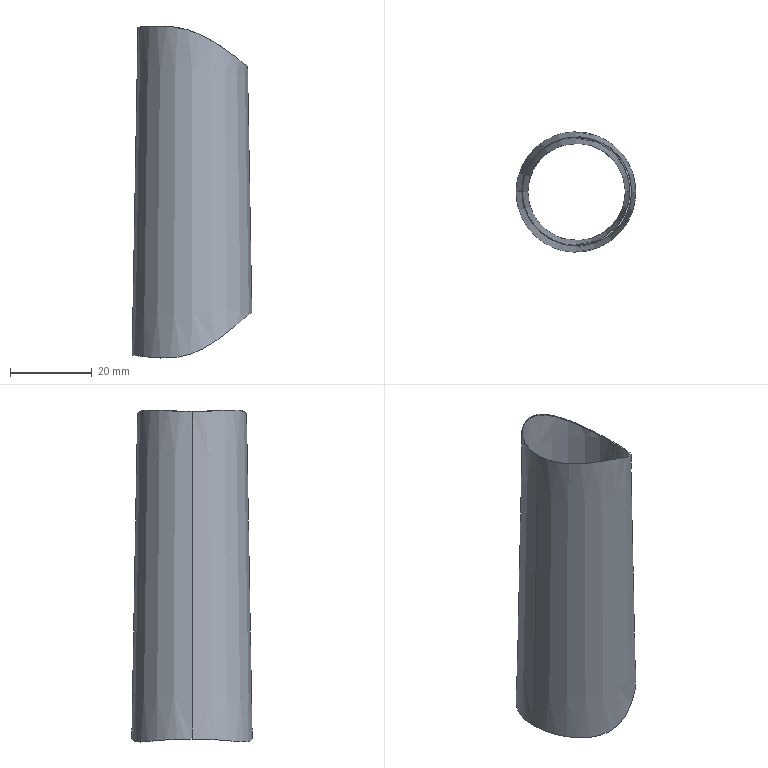Part | STEP file | PRT0001_68_22 | 1 solid | 6 faces | box 29.224 x 29.394 x 81.102 mm | volume 9192 mm3 | cone 4 | other 2